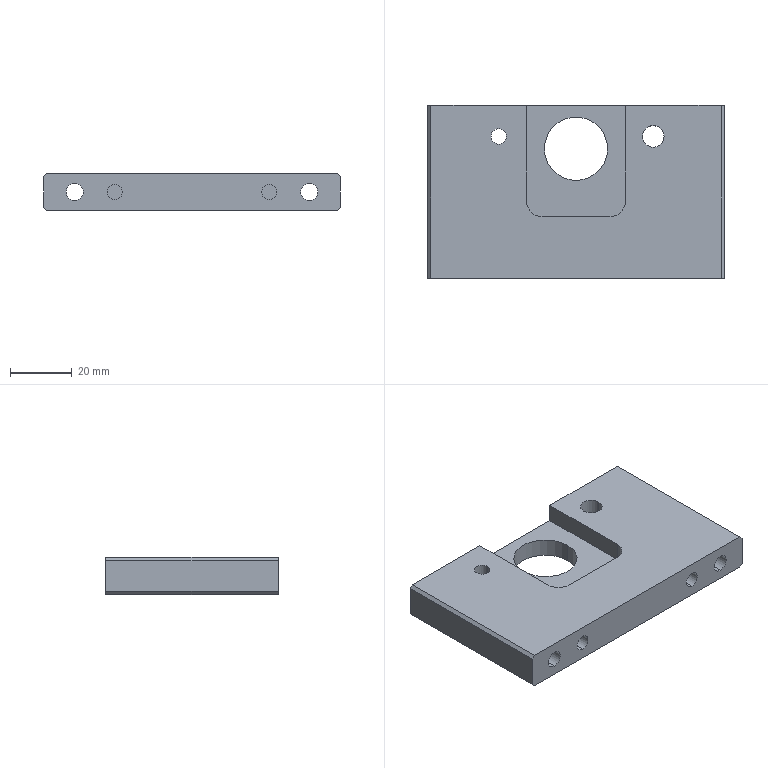Part | STEP file | PN_0081 transport cylinder mounting plate | 1 solid | 38 faces | box 96 x 56 x 12 mm | volume 48456 mm3 | cylinder 20 | plane 18 | commonest cylinder face diameters 5 x6 10 x6 5.5 x4 7 x2 20.5 x2